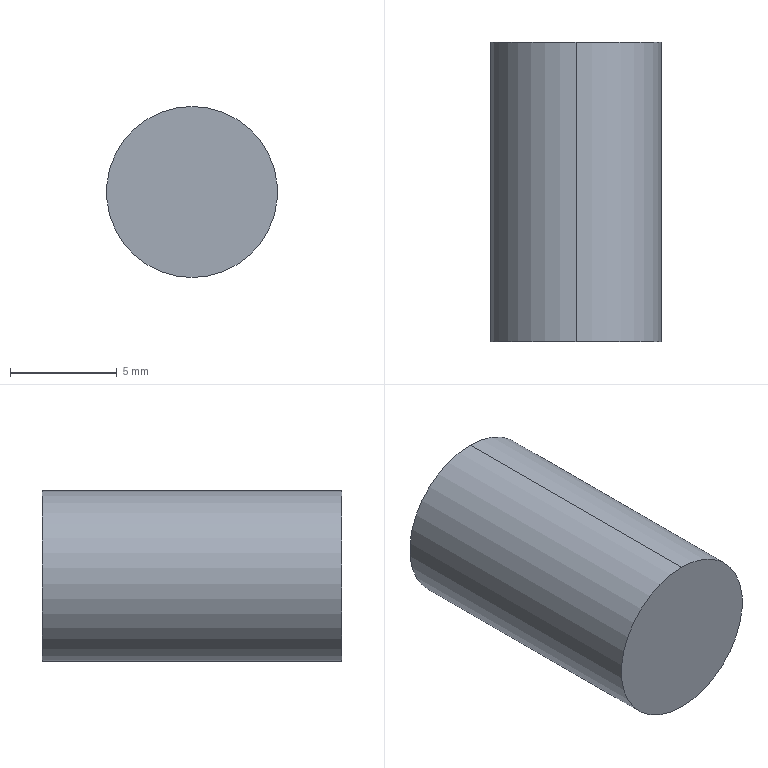Part | SolidWorks | features BaseBody 1 | 1 solid | 4 faces | box 8 x 14 x 8 mm | volume 703.717 mm3 | cylinder 2 | plane 2 | commonest cylinder face diameters 8 x2
STEP:
#1=CARTESIAN_POINT('',(0.,14.,-4.));
#2=VERTEX_POINT('',#1);
#3=CARTESIAN_POINT('',(0.,14.,4.));
#4=VERTEX_POINT('',#3);
#5=CARTESIAN_POINT('',(0.,14.,0.));
#6=DIRECTION('',(0.,-1.,0.));
#7=DIRECTION('',(0.,0.,-1.));
#8=AXIS2_PLACEMENT_3D('',#5,#6,#7);
#9=CIRCLE('',#8,4.);
#10=EDGE_CURVE('',#2,#4,#9,.T.);
#11=ORIENTED_EDGE('',*,*,#10,.T.);
#12=CARTESIAN_POINT('',(0.,0.,4.));
#13=VERTEX_POINT('',#12);
#14=CARTESIAN_POINT('',(0.,14.,4.));
#15=DIRECTION('',(0.,-1.,0.));
#16=VECTOR('',#15,1000.);
#17=LINE('',#14,#16);
#18=EDGE_CURVE('',#4,#13,#17,.T.);
#19=ORIENTED_EDGE('',*,*,#18,.T.);
#20=CARTESIAN_POINT('',(0.,0.,-4.));
#21=VERTEX_POINT('',#20);
#22=CARTESIAN_POINT('',(0.,0.,0.));
#23=DIRECTION('',(0.,1.,0.));
#24=DIRECTION('',(0.,0.,-1.));
#25=AXIS2_PLACEMENT_3D('',#22,#23,#24);
#26=CIRCLE('',#25,4.);
#27=EDGE_CURVE('',#13,#21,#26,.T.);
#28=ORIENTED_EDGE('',*,*,#27,.T.);
#29=CARTESIAN_POINT('',(0.,14.,-4.));
#30=DIRECTION('',(0.,-1.,0.));
#31=VECTOR('',#30,1000.);
#32=LINE('',#29,#31);
#33=EDGE_CURVE('',#2,#21,#32,.T.);
#34=ORIENTED_EDGE('',*,*,#33,.F.);
#35=EDGE_LOOP('',(#11,#19,#28,#34));
#36=FACE_OUTER_BOUND('',#35,.T.);
#37=CARTESIAN_POINT('',(0.,14.,0.));
#38=DIRECTION('',(0.,-1.,0.));
#39=DIRECTION('',(0.,0.,-1.));
#40=AXIS2_PLACEMENT_3D('',#37,#38,#39);
#41=CYLINDRICAL_SURFACE('',#40,4.);
#42=ADVANCED_FACE('',(#36),#41,.T.);
#43=ORIENTED_EDGE('',*,*,#18,.F.);
#44=CARTESIAN_POINT('',(0.,14.,0.));
#45=DIRECTION('',(0.,-1.,0.));
#46=DIRECTION('',(0.,0.,-1.));
#47=AXIS2_PLACEMENT_3D('',#44,#45,#46);
#48=CIRCLE('',#47,4.);
#49=EDGE_CURVE('',#4,#2,#48,.T.);
#50=ORIENTED_EDGE('',*,*,#49,.T.);
#51=ORIENTED_EDGE('',*,*,#33,.T.);
#52=CARTESIAN_POINT('',(0.,0.,0.));
#53=DIRECTION('',(0.,1.,0.));
#54=DIRECTION('',(0.,0.,-1.));
#55=AXIS2_PLACEMENT_3D('',#52,#53,#54);
#56=CIRCLE('',#55,4.);
#57=EDGE_CURVE('',#21,#13,#56,.T.);
#58=ORIENTED_EDGE('',*,*,#57,.T.);
#59=EDGE_LOOP('',(#43,#50,#51,#58));
#60=FACE_OUTER_BOUND('',#59,.T.);
#61=CARTESIAN_POINT('',(0.,14.,0.));
#62=DIRECTION('',(0.,-1.,0.));
#63=DIRECTION('',(0.,0.,-1.));
#64=AXIS2_PLACEMENT_3D('',#61,#62,#63);
#65=CYLINDRICAL_SURFACE('',#64,4.);
#66=ADVANCED_FACE('',(#60),#65,.T.);
#67=ORIENTED_EDGE('',*,*,#57,.F.);
#68=ORIENTED_EDGE('',*,*,#27,.F.);
#69=EDGE_LOOP('',(#67,#68));
#70=FACE_OUTER_BOUND('',#69,.T.);
#71=CARTESIAN_POINT('',(0.,0.,0.));
#72=DIRECTION('',(0.,1.,0.));
#73=DIRECTION('',(0.,0.,1.));
#74=AXIS2_PLACEMENT_3D('',#71,#72,#73);
#75=PLANE('',#74);
#76=ADVANCED_FACE('',(#70),#75,.F.);
#77=ORIENTED_EDGE('',*,*,#10,.F.);
#78=ORIENTED_EDGE('',*,*,#49,.F.);
#79=EDGE_LOOP('',(#77,#78));
#80=FACE_OUTER_BOUND('',#79,.T.);
#81=CARTESIAN_POINT('',(0.,14.,0.));
#82=DIRECTION('',(0.,1.,0.));
#83=DIRECTION('',(0.,0.,1.));
#84=AXIS2_PLACEMENT_3D('',#81,#82,#83);
#85=PLANE('',#84);
#86=ADVANCED_FACE('',(#80),#85,.T.);
#87=CLOSED_SHELL('',(#42,#66,#76,#86));
#88=MANIFOLD_SOLID_BREP('',#87);
#89=CARTESIAN_POINT('',(0.,0.,0.));
#90=DIRECTION('',(0.,0.,1.));
#91=DIRECTION('',(1.,0.,0.));
#92=AXIS2_PLACEMENT_3D('',#89,#90,#91);
#93=(LENGTH_UNIT()NAMED_UNIT(*)SI_UNIT(.MILLI.,.METRE.));
#94=UNCERTAINTY_MEASURE_WITH_UNIT(LENGTH_MEASURE(0.00001),#93,'','');
#95=(NAMED_UNIT(*)PLANE_ANGLE_UNIT()SI_UNIT($,.RADIAN.));
#96=(NAMED_UNIT(*)SI_UNIT($,.STERADIAN.)SOLID_ANGLE_UNIT());
#97=(GEOMETRIC_REPRESENTATION_CONTEXT(3)GLOBAL_UNCERTAINTY_ASSIGNED_CONTEXT((#94))GLOBAL_UNIT_ASSIGNED_CONTEXT((#93,#95,#96))REPRESENTATION_CONTEXT('',''));
#98=ADVANCED_BREP_SHAPE_REPRESENTATION('',(#88,#92),#97);